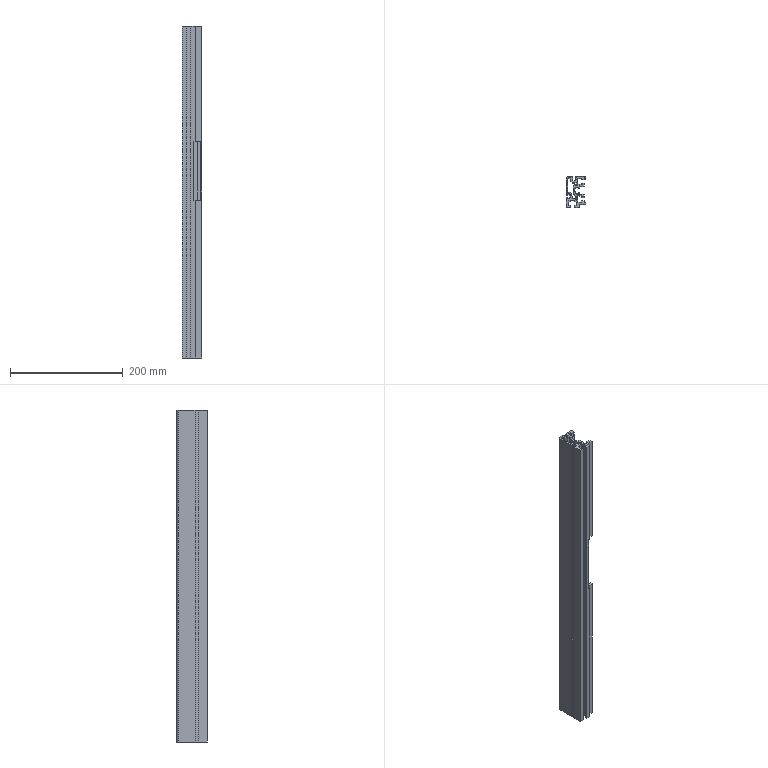Part | STEP file | Conveyor front chain guide groove L590 | 1 solid | 174 faces | box 35 x 55 x 590 mm | volume 449690 mm3 | plane 128 | cylinder 37 | cone 9 | commonest cylinder face diameters 2.5 x9 2 x8 6.5 x6 2.3 x4 11 x4 24 x4